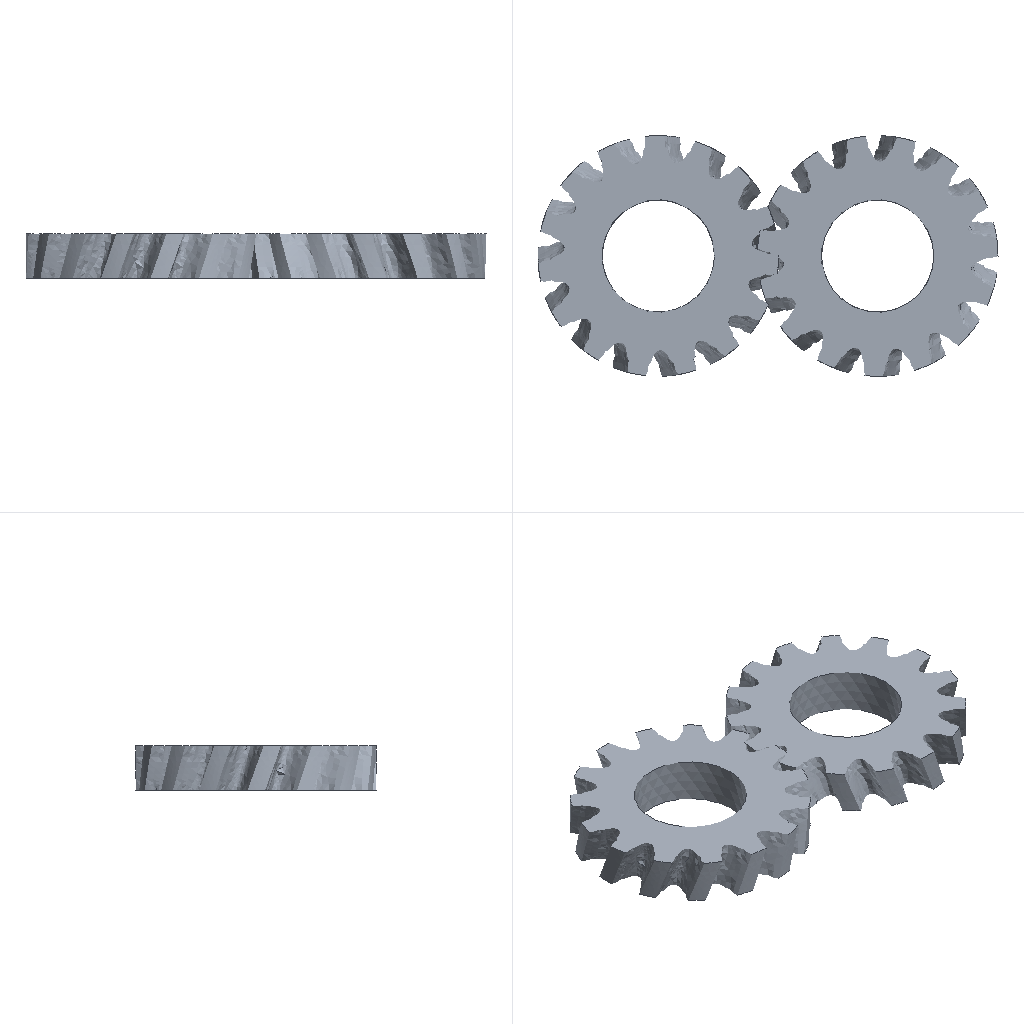Simulation study | ansys workbench
Set-up summary:
category,name,step,type,value,unit,region
solver,ansys_mapdl
solver,version,,,16.0
solver,version,,,16.0
units,MPA,,stated
analysis,deck1,,transient,transient
load_step,requested,,,2
analysis,nlgeom,,,True
mesh,nodes,,,51988
mesh,elements,,,41332
element_type,ANSYS 187 (type 1),,solid,11470
element_type,ANSYS 187 (type 2),,solid,14800
element_type,ANSYS 174 (type 3),,contact,7330
element_type,ANSYS 170 (type 4),,target,7330
element_type,ANSYS 174 (type 5),,contact,200
element_type,ANSYS 170 (type 6),,target,0
element_type,ANSYS 174 (type 7),,contact,200
element_type,ANSYS 170 (type 8),,target,0
element_type,ANSYS 184 (type 9),,mpc,1
element_type,ANSYS 184 (type 10),,mpc,1
load,load commands in deck,,count,1
bc,support commands in deck,,count,1
named_set,SELECTION,,component
named_set,SELECTION_2,,component
named_set,_ELMISC,,component
analysis,deck2,,static,static
load_step,requested,,,1
analysis,nlgeom,,,False
mesh,nodes,,,51988
mesh,elements,,,41332
element_type,ANSYS 187 (type 1),,solid,11470
element_type,ANSYS 187 (type 2),,solid,14800
element_type,ANSYS 174 (type 3),,contact,7330
element_type,ANSYS 170 (type 4),,target,7330
element_type,ANSYS 174 (type 5),,contact,200
element_type,ANSYS 170 (type 6),,target,0
element_type,ANSYS 174 (type 7),,contact,200
element_type,ANSYS 170 (type 8),,target,0
element_type,ANSYS 184 (type 9),,mpc,1
element_type,ANSYS 184 (type 10),,mpc,1
element_type,ANSYS 14 (type 11),,spring,0
load,load commands in deck,,count,2
bc,support commands in deck,,count,2
named_set,SELECTION,,component
named_set,SELECTION_2,,component
named_set,_ELMISC,,component
material,1,,in results
material,2,,in results
material,1,,in results
material,2,,in results
check,setup vs results,,match,"results also hold 8 node(s) and 2 element(s) the deck makes with ['EN']; those were not compared; 2 setup node(s) no element uses are not in the results (e.g. [51985, 51987])"
check,setup vs results,,match,"results also hold 56 node(s) and 50 element(s) the deck makes with ['E', 'EN', 'N']; those were not compared; 2 setup node(s) no element uses are not in the results (e.g. [51985, 51987])"
Results summary:
result,analysis,,,static
result,last_loadstep,,,2
result,primary field,,,displacement
result,reaction total,23,FX,0.0,N
result,reaction total,23,FY,0.0,N
result,reaction total,23,FZ,0.0,N
result,mass,,,0.000213,"NMM: mm, ton, N, s, mV, mA, degC"
result,analysis,,,static
result,last_loadstep,,,1
result,primary field,,,displacement
result,reaction total,5,FX,4e-06,N
result,reaction total,5,FY,-1e-06,N
result,reaction total,5,FZ,3e-06,N
result,mass,,,0.000213,"NMM: mm, ton, N, s, mV, mA, degC"